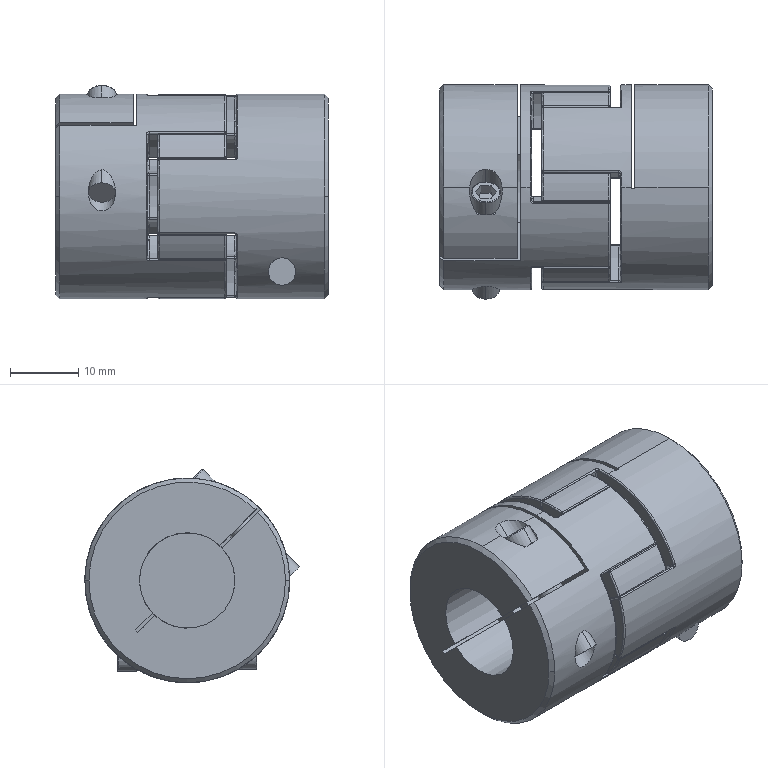Part | SolidWorks | features BaseBody 3 | 3 solids | 406 faces | box 40 x 31.403 x 31.299 mm | volume 20689 mm3 | spline 216 | cylinder 134 | plane 50 | cone 6 | commonest cylinder face diameters 0.4 x58 18 x36 30 x13 4 x9 14 x7 14.4 x4